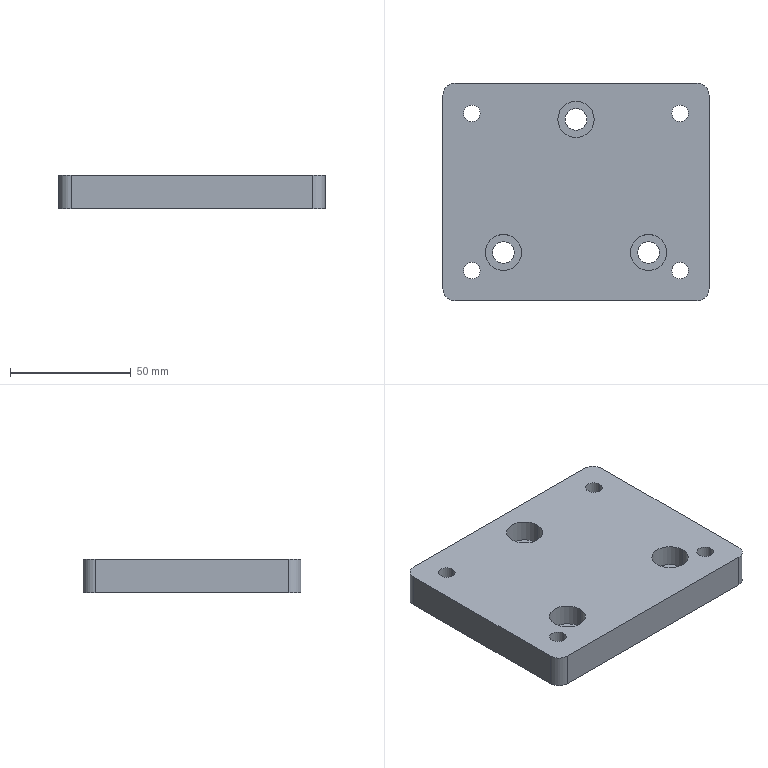Part | STEP file | Caster mounting plate | 1 solid | 33 faces | box 110 x 90 x 14 mm | volume 130540 mm3 | cylinder 24 | plane 9 | commonest cylinder face diameters 6.8 x8 9 x6 15 x6 10 x4